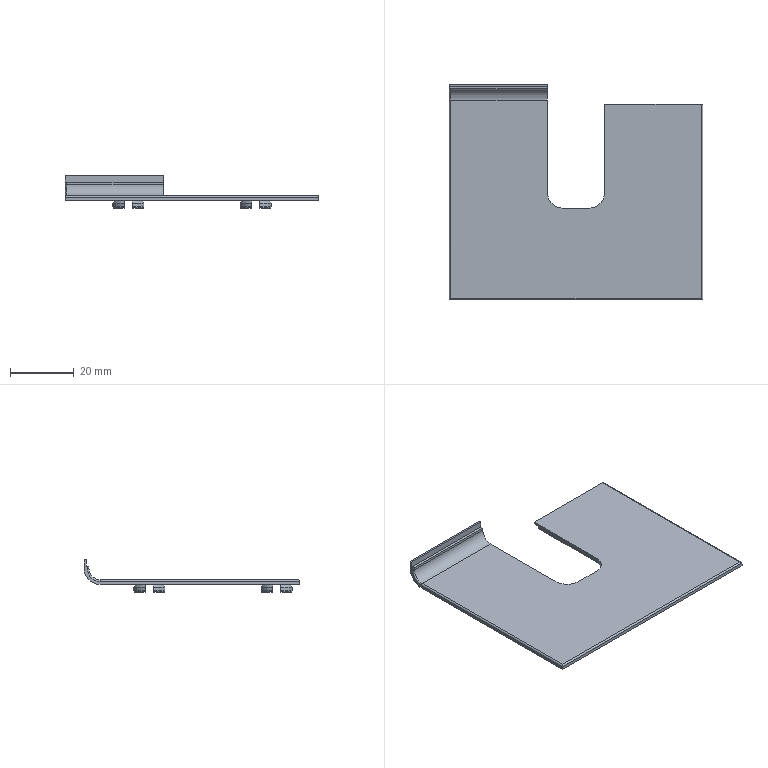Part | STEP file | 00371716_ABDECKKAPPE_HMB-....2 | 1 solid | 337 faces | box 79.8 x 67.8 x 10.238 mm | volume 5792 mm3 | spline 129 | cone 80 | plane 68 | cylinder 60 | commonest cylinder face diameters 9.1 x16 10.1 x16 3 x13 16 x7 1 x4 10 x3